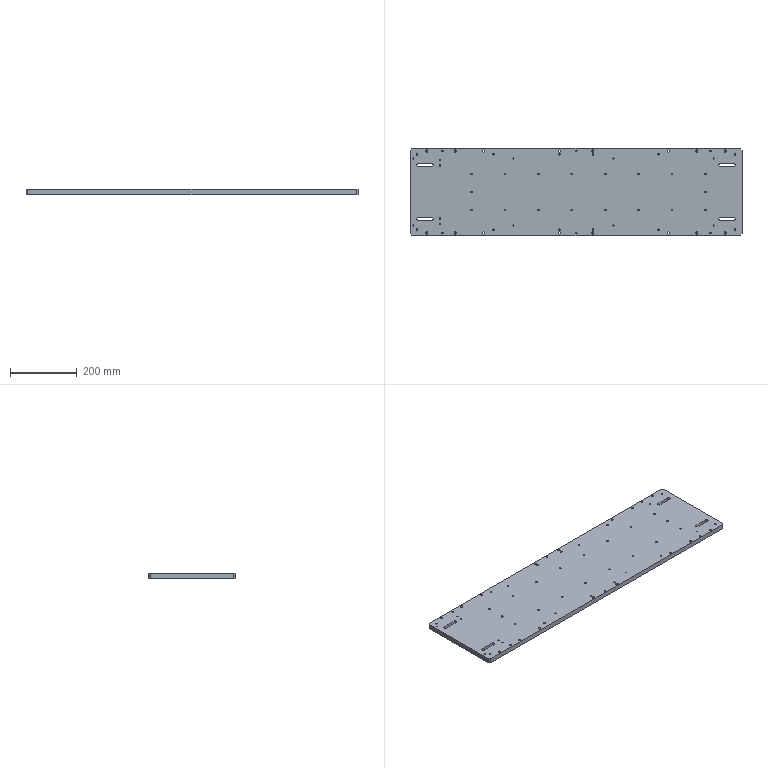CAM job | NX | 3-axis milling, drilling | part box 995 x 261 x 15 mm | stock box 1000 x 266 x 15 mm
Tools:
number,name,description,diameter,corner_radius,flute_length,length,flutes
6,D6,平底铣刀-粗,6.0,0.0,25.0,75.0,2
9,D10,平底铣刀-粗,10.0,0.0,35.0,75.0,2
17,D2-J,平底铣刀-精,2.0,0.0,50.0,75.0,2
20,D3-J,平底铣刀-精,3.0,0.0,50.0,75.0,2
11,D4-J,平底铣刀-精,4.0,0.0,50.0,75.0,2
7,D6-J,平底铣刀-精,6.0,0.0,25.0,75.0,2
2,D6_CHAMFERMILL,倒角刀,6.0,0.0,3.0,25.0,2
13,ZT3.4,钻头,3.4,0.0,35.0,50.0,2
18,ZT4.8,钻头,4.8,0.0,35.0,50.0,2
15,ZT5.1,钻头,5.1,0.0,35.0,50.0,2
19,ZT5.8,钻头,5.8,0.0,35.0,50.0,2
16,ZT6.8,钻头,6.8,0.0,35.0,50.0,2
14,ZT4.3,Drilling Tool,4.3,0.0,50.0,75.0,4
Operations:
program,operation,operation_type,tool,method,geometry_group,spindle_rpm,surface_speed,feed_per_tooth,feed_cut,feed_plunge,cut_length_mm,path_length_mm,cut_time_min,machine_time_min
B,SPOT_2,Operation,D6_CHAMFERMILL,METHOD,W-B,3000.0,56.549,0.0333,200.0,0.0,160.0,3924.809,0.8,1.177
B,MILLCHAMFER_4,PlanarMilling,D6_CHAMFERMILL,METHOD,W-B,8000.0,150.796,0.0375,600.0,100.0,307.147,3442.359,0.5119,0.8254
B,DRILLCHAMFER_4,Operation,D6_CHAMFERMILL,METHOD,W-B,8000.0,150.796,0.0625,1000.0,0.0,41.6,1908.334,0.0416,0.2283
B,DRILLCHAMFER_5,Operation,D6_CHAMFERMILL,METHOD,W-B,8000.0,150.796,0.0625,1000.0,0.0,22.8,346.186,0.0228,0.0551
B,DRILLCHAMFER_DJ10_1,Operation,D6_CHAMFERMILL,METHOD,W-B,8000.0,150.796,0.0625,1000.0,0.0,104.4,2502.502,0.1044,0.3442
B,MILLCHAMFER_6,PlanarMilling,D6_CHAMFERMILL,METHOD,W-B,8000.0,150.796,0.0375,600.0,100.0,37.911,941.513,0.0632,0.1535
B,MILLCHAMFER_7,PlanarMilling,D6_CHAMFERMILL,METHOD,W-B,8000.0,150.796,0.0375,600.0,100.0,500.389,4168.243,0.834,1.201
B,C0.3_CLOSEDCONTOURCHAMFER6X45L_COPY,PlanarMilling,D6_CHAMFERMILL,CLIMBFACE_CHAMFER-DEPTH0-STEPG,W-B,7000.0,131.0,0.1071,1500.0,100.0,476.438,2098.187,0.3176,0.4798
B,C0.3_OPENCONTOURCHAMFER6X45L_COPY,PlanarMilling,D6_CHAMFERMILL,CLIMBFACE_CHAMFER-DEPTH0-STEPG,W-B,7000.0,131.0,0.1071,1500.0,100.0,554.432,1730.179,0.3696,0.4872
A,SPOT,Operation,D6_CHAMFERMILL,METHOD,W-A,3000.0,56.549,0.0333,200.0,0.0,160.0,3887.452,0.8,1.173
A,DRILL,Operation,ZT3.4,METHOD,W-A,3500.0,36.285,0.0143,100.0,0.0,124.0,2019.015,1.24,1.429
A,DRILL_2,Operation,ZT4.3,METHOD,W-A,3000.0,39.584,0.0167,100.0,0.0,62.0,378.066,0.62,0.6516
A,DRILL_3,Operation,ZT4.8,METHOD,W-A,3000.0,45.239,0.025,150.0,0.0,282.6,2784.176,1.884,2.134
A,DRILL_4,Operation,ZT5.1,METHOD,W-A,2800.0,44.862,0.0214,120.0,0.0,251.2,2085.475,2.093,2.277
A,DRILL_5,Operation,ZT5.8,METHOD,W-A,3000.0,54.664,0.025,150.0,0.0,31.4,823.801,0.2093,0.2886
A,DRILL_6,Operation,ZT6.8,METHOD,W-A,2500.0,53.407,0.024,120.0,0.0,251.2,2611.468,2.093,2.329
A,FLOORWALL_SPIRALFINISH-MID_COPY,VolumeBased25DMillingOperation,D2-J,SPIRALFINISH-DEPTHK-STEPG,W-A,8000.0,50.264,0.0375,600.0,100.0,1531.629,3822.536,2.553,2.782
A,FLOORWALL_SPIRALFINISH-MID_COPY_COPY,VolumeBased25DMillingOperation,D3-J,SPIRALFINISH-DEPTHK-STEPG,W-A,8000.0,50.264,0.0375,600.0,100.0,710.866,1194.843,1.185,1.233
A,FLOORWALL_SPIRALFINISH-MID_COPY_COPY_COPY_COPY,VolumeBased25DMillingOperation,D3-J,SPIRALFINISH-DEPTHK-STEPG,W-A,8000.0,75.398,0.05,800.0,100.0,3459.239,6145.895,4.324,4.593
A,FLOORWALL_SPIRALFINISH-MID_COPY_COPY_COPY_COPY_COPY,VolumeBased25DMillingOperation,D4-J,SPIRALFINISH-DEPTHK-STEPG,W-A,8000.0,75.398,0.05,800.0,100.0,4547.794,7738.462,5.685,6.004
A,THRUSLOT_ROUGH_1,VolumeBased25DMillingOperation,D6,METHOD,W-A,6000.0,113.0,0.2083,2500.0,100.0,11628.111,13148.417,4.651,4.803
A,SLOT_FINISH_1,VolumeBased25DMillingOperation,D6-J,METHOD,W-A,6000.0,113.0,0.0667,600.0,100.0,1123.837,2797.377,1.873,2.04
A,PROFILE_ROUGH_2,VolumeBased25DMillingOperation,D10,METHOD,W-A,6000.0,188.0,0.25,4000.0,80.0,78503.685,78576.685,19.626,19.633
A,SELECTSOLIDONLY,SurfaceContour,D6_CHAMFERMILL,METHOD,W-A,6000.0,113.0,0.125,1200.0,100.0,2962.597,4918.587,2.469,2.664
A,DRILLCHAMFER_1,Operation,D6_CHAMFERMILL,METHOD,W-A,5000.0,94.248,0.015,150.0,0.0,41.6,1868.334,0.2773,0.46
A,DRILLCHAMFER_2,Operation,D6_CHAMFERMILL,METHOD,W-A,5000.0,94.248,0.015,150.0,0.0,22.8,306.186,0.152,0.1803
A,DRILLCHAMFER_3,Operation,D6_CHAMFERMILL,METHOD,W-A,5000.0,94.248,0.015,150.0,0.0,104.4,2462.502,0.696,0.9318
A,MILLCHAMFER_1,PlanarMilling,D6_CHAMFERMILL,METHOD,W-A,6000.0,113.097,0.05,600.0,100.0,284.714,2789.324,0.4745,0.725
A,MILLCHAMFER_2,PlanarMilling,D6_CHAMFERMILL,METHOD,W-A,6000.0,113.097,0.05,600.0,100.0,37.911,861.513,0.0632,0.1455
A,MILLCHAMFER_3,PlanarMilling,D6_CHAMFERMILL,METHOD,W-A,6000.0,113.097,0.05,600.0,100.0,382.645,3409.438,0.6377,0.9404
A,FLOORWALL_SPIRALFINISH-MID_COPY_COPY_COPY,VolumeBased25DMillingOperation,D3-J,SPIRALFINISH-DEPTHK-STEPG,W-A,8000.0,75.398,0.0187,300.0,100.0,3751.796,7213.901,12.506,12.852
A,FLOORWALL_SPIRALFINISH-MID_COPY_COPY_COPY_COPY_1,VolumeBased25DMillingOperation,D3-J,SPIRALFINISH-DEPTHK-STEPG,W-A,8000.0,75.398,0.0187,300.0,100.0,611.265,1458.89,2.038,2.122
A,PROFILE_SEMIFINISH_2,VolumeBased25DMillingOperation,D6-J,METHOD,W-A,6000.0,113.0,0.0833,1000.0,100.0,5048.1,5212.12,5.048,5.064
A,PROFILE_FINISH_2,VolumeBased25DMillingOperation,D6-J,METHOD,W-A,6000.0,113.0,0.0833,1000.0,100.0,2523.85,2612.45,2.524,2.533